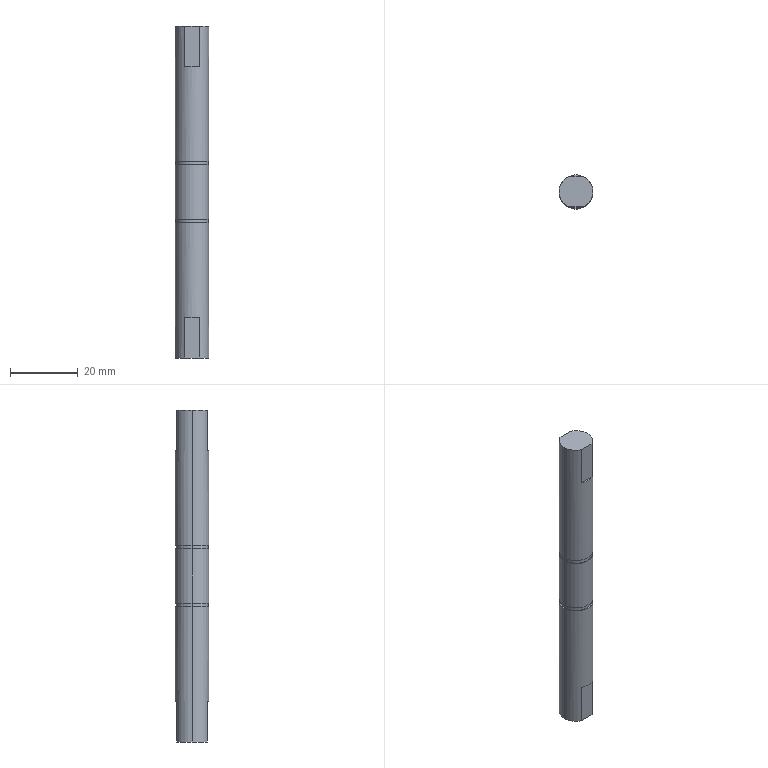Part | SolidWorks | features ICE 2, MirrorPattern 2, Extrusion 1, RefAxis 1 | 1 solid | 24 faces | box 10 x 10 x 98 mm | volume 7613 mm3 | plane 14 | cylinder 10 | commonest cylinder face diameters 10 x6 9.6 x4
STEP:
#1=CARTESIAN_POINT('',(4.8,0.,-9.1));
#2=VERTEX_POINT('',#1);
#3=CARTESIAN_POINT('',(-4.8,0.,-9.1));
#4=VERTEX_POINT('',#3);
#5=CARTESIAN_POINT('',(0.,0.,-9.1));
#6=DIRECTION('',(0.,0.,1.));
#7=DIRECTION('',(1.,0.,0.));
#8=AXIS2_PLACEMENT_3D('',#5,#6,#7);
#9=CIRCLE('',#8,4.8);
#10=EDGE_CURVE('',#2,#4,#9,.T.);
#11=ORIENTED_EDGE('',*,*,#10,.T.);
#12=CARTESIAN_POINT('',(-4.8,0.,-8.));
#13=VERTEX_POINT('',#12);
#14=CARTESIAN_POINT('',(-4.8,0.,-9.1));
#15=DIRECTION('',(0.,0.,1.));
#16=VECTOR('',#15,1000.);
#17=LINE('',#14,#16);
#18=EDGE_CURVE('',#4,#13,#17,.T.);
#19=ORIENTED_EDGE('',*,*,#18,.T.);
#20=CARTESIAN_POINT('',(4.8,0.,-8.));
#21=VERTEX_POINT('',#20);
#22=CARTESIAN_POINT('',(0.,0.,-8.));
#23=DIRECTION('',(0.,0.,1.));
#24=DIRECTION('',(1.,0.,0.));
#25=AXIS2_PLACEMENT_3D('',#22,#23,#24);
#26=CIRCLE('',#25,4.8);
#27=EDGE_CURVE('',#21,#13,#26,.T.);
#28=ORIENTED_EDGE('',*,*,#27,.F.);
#29=CARTESIAN_POINT('',(4.8,0.,-9.1));
#30=DIRECTION('',(0.,0.,1.));
#31=VECTOR('',#30,1000.);
#32=LINE('',#29,#31);
#33=EDGE_CURVE('',#2,#21,#32,.T.);
#34=ORIENTED_EDGE('',*,*,#33,.F.);
#35=EDGE_LOOP('',(#11,#19,#28,#34));
#36=FACE_OUTER_BOUND('',#35,.T.);
#37=CARTESIAN_POINT('',(0.,0.,-9.1));
#38=DIRECTION('',(0.,0.,1.));
#39=DIRECTION('',(1.,0.,0.));
#40=AXIS2_PLACEMENT_3D('',#37,#38,#39);
#41=CYLINDRICAL_SURFACE('',#40,4.8);
#42=ADVANCED_FACE('',(#36),#41,.T.);
#43=CARTESIAN_POINT('',(4.8,0.,9.1));
#44=VERTEX_POINT('',#43);
#45=CARTESIAN_POINT('',(-4.8,0.,9.1));
#46=VERTEX_POINT('',#45);
#47=CARTESIAN_POINT('',(0.,0.,9.1));
#48=DIRECTION('',(0.,0.,1.));
#49=DIRECTION('',(1.,0.,0.));
#50=AXIS2_PLACEMENT_3D('',#47,#48,#49);
#51=CIRCLE('',#50,4.8);
#52=EDGE_CURVE('',#44,#46,#51,.T.);
#53=ORIENTED_EDGE('',*,*,#52,.F.);
#54=CARTESIAN_POINT('',(4.8,0.,8.));
#55=VERTEX_POINT('',#54);
#56=CARTESIAN_POINT('',(4.8,0.,9.1));
#57=DIRECTION('',(0.,0.,-1.));
#58=VECTOR('',#57,1000.);
#59=LINE('',#56,#58);
#60=EDGE_CURVE('',#44,#55,#59,.T.);
#61=ORIENTED_EDGE('',*,*,#60,.T.);
#62=CARTESIAN_POINT('',(-4.8,0.,8.));
#63=VERTEX_POINT('',#62);
#64=CARTESIAN_POINT('',(0.,0.,8.));
#65=DIRECTION('',(0.,0.,1.));
#66=DIRECTION('',(1.,0.,0.));
#67=AXIS2_PLACEMENT_3D('',#64,#65,#66);
#68=CIRCLE('',#67,4.8);
#69=EDGE_CURVE('',#55,#63,#68,.T.);
#70=ORIENTED_EDGE('',*,*,#69,.T.);
#71=CARTESIAN_POINT('',(-4.8,0.,9.1));
#72=DIRECTION('',(0.,0.,-1.));
#73=VECTOR('',#72,1000.);
#74=LINE('',#71,#73);
#75=EDGE_CURVE('',#46,#63,#74,.T.);
#76=ORIENTED_EDGE('',*,*,#75,.F.);
#77=EDGE_LOOP('',(#53,#61,#70,#76));
#78=FACE_OUTER_BOUND('',#77,.T.);
#79=CARTESIAN_POINT('',(0.,0.,9.1));
#80=DIRECTION('',(0.,0.,-1.));
#81=DIRECTION('',(-1.,0.,0.));
#82=AXIS2_PLACEMENT_3D('',#79,#80,#81);
#83=CYLINDRICAL_SURFACE('',#82,4.8);
#84=ADVANCED_FACE('',(#78),#83,.T.);
#85=CARTESIAN_POINT('',(5.,0.,49.));
#86=VERTEX_POINT('',#85);
#87=CARTESIAN_POINT('',(2.179,4.5,49.));
#88=VERTEX_POINT('',#87);
#89=CARTESIAN_POINT('',(0.,0.,49.));
#90=DIRECTION('',(0.,0.,1.));
#91=DIRECTION('',(1.,0.,0.));
#92=AXIS2_PLACEMENT_3D('',#89,#90,#91);
#93=CIRCLE('',#92,5.);
#94=EDGE_CURVE('',#86,#88,#93,.T.);
#95=ORIENTED_EDGE('',*,*,#94,.F.);
#96=CARTESIAN_POINT('',(5.,0.,9.1));
#97=VERTEX_POINT('',#96);
#98=CARTESIAN_POINT('',(5.,0.,49.));
#99=DIRECTION('',(0.,0.,-1.));
#100=VECTOR('',#99,1000.);
#101=LINE('',#98,#100);
#102=EDGE_CURVE('',#86,#97,#101,.T.);
#103=ORIENTED_EDGE('',*,*,#102,.T.);
#104=CARTESIAN_POINT('',(-5.,0.,9.1));
#105=VERTEX_POINT('',#104);
#106=CARTESIAN_POINT('',(0.,0.,9.1));
#107=DIRECTION('',(0.,0.,1.));
#108=DIRECTION('',(1.,0.,0.));
#109=AXIS2_PLACEMENT_3D('',#106,#107,#108);
#110=CIRCLE('',#109,5.);
#111=EDGE_CURVE('',#97,#105,#110,.T.);
#112=ORIENTED_EDGE('',*,*,#111,.T.);
#113=CARTESIAN_POINT('',(-5.,0.,49.));
#114=VERTEX_POINT('',#113);
#115=CARTESIAN_POINT('',(-5.,0.,49.));
#116=DIRECTION('',(0.,0.,-1.));
#117=VECTOR('',#116,1000.);
#118=LINE('',#115,#117);
#119=EDGE_CURVE('',#114,#105,#118,.T.);
#120=ORIENTED_EDGE('',*,*,#119,.F.);
#121=CARTESIAN_POINT('',(-2.179,4.5,49.));
#122=VERTEX_POINT('',#121);
#123=CARTESIAN_POINT('',(0.,0.,49.));
#124=DIRECTION('',(0.,0.,1.));
#125=DIRECTION('',(1.,0.,0.));
#126=AXIS2_PLACEMENT_3D('',#123,#124,#125);
#127=CIRCLE('',#126,5.);
#128=EDGE_CURVE('',#122,#114,#127,.T.);
#129=ORIENTED_EDGE('',*,*,#128,.F.);
#130=CARTESIAN_POINT('',(-2.179,4.5,37.));
#131=VERTEX_POINT('',#130);
#132=CARTESIAN_POINT('',(-2.179,4.5,37.));
#133=DIRECTION('',(0.,0.,1.));
#134=VECTOR('',#133,1000.);
#135=LINE('',#132,#134);
#136=EDGE_CURVE('',#131,#122,#135,.T.);
#137=ORIENTED_EDGE('',*,*,#136,.F.);
#138=CARTESIAN_POINT('',(2.179,4.5,37.));
#139=VERTEX_POINT('',#138);
#140=CARTESIAN_POINT('',(0.,0.,37.));
#141=DIRECTION('',(0.,0.,1.));
#142=DIRECTION('',(1.,0.,0.));
#143=AXIS2_PLACEMENT_3D('',#140,#141,#142);
#144=CIRCLE('',#143,5.);
#145=EDGE_CURVE('',#139,#131,#144,.T.);
#146=ORIENTED_EDGE('',*,*,#145,.F.);
#147=CARTESIAN_POINT('',(2.179,4.5,37.));
#148=DIRECTION('',(0.,0.,1.));
#149=VECTOR('',#148,1000.);
#150=LINE('',#147,#149);
#151=EDGE_CURVE('',#139,#88,#150,.T.);
#152=ORIENTED_EDGE('',*,*,#151,.T.);
#153=EDGE_LOOP('',(#95,#103,#112,#120,#129,#137,#146,#152));
#154=FACE_OUTER_BOUND('',#153,.T.);
#155=CARTESIAN_POINT('',(0.,0.,49.));
#156=DIRECTION('',(0.,0.,-1.));
#157=DIRECTION('',(-1.,0.,0.));
#158=AXIS2_PLACEMENT_3D('',#155,#156,#157);
#159=CYLINDRICAL_SURFACE('',#158,5.);
#160=ADVANCED_FACE('',(#154),#159,.T.);
#161=CARTESIAN_POINT('',(5.,0.,8.));
#162=VERTEX_POINT('',#161);
#163=CARTESIAN_POINT('',(-5.,0.,8.));
#164=VERTEX_POINT('',#163);
#165=CARTESIAN_POINT('',(0.,0.,8.));
#166=DIRECTION('',(0.,0.,1.));
#167=DIRECTION('',(1.,0.,0.));
#168=AXIS2_PLACEMENT_3D('',#165,#166,#167);
#169=CIRCLE('',#168,5.);
#170=EDGE_CURVE('',#162,#164,#169,.T.);
#171=ORIENTED_EDGE('',*,*,#170,.F.);
#172=CARTESIAN_POINT('',(5.,0.,-8.));
#173=VERTEX_POINT('',#172);
#174=CARTESIAN_POINT('',(5.,0.,49.));
#175=DIRECTION('',(0.,0.,-1.));
#176=VECTOR('',#175,1000.);
#177=LINE('',#174,#176);
#178=EDGE_CURVE('',#162,#173,#177,.T.);
#179=ORIENTED_EDGE('',*,*,#178,.T.);
#180=CARTESIAN_POINT('',(-5.,0.,-8.));
#181=VERTEX_POINT('',#180);
#182=CARTESIAN_POINT('',(0.,0.,-8.));
#183=DIRECTION('',(0.,0.,1.));
#184=DIRECTION('',(1.,0.,0.));
#185=AXIS2_PLACEMENT_3D('',#182,#183,#184);
#186=CIRCLE('',#185,5.);
#187=EDGE_CURVE('',#173,#181,#186,.T.);
#188=ORIENTED_EDGE('',*,*,#187,.T.);
#189=CARTESIAN_POINT('',(-5.,0.,49.));
#190=DIRECTION('',(0.,0.,-1.));
#191=VECTOR('',#190,1000.);
#192=LINE('',#189,#191);
#193=EDGE_CURVE('',#164,#181,#192,.T.);
#194=ORIENTED_EDGE('',*,*,#193,.F.);
#195=EDGE_LOOP('',(#171,#179,#188,#194));
#196=FACE_OUTER_BOUND('',#195,.T.);
#197=CARTESIAN_POINT('',(0.,0.,49.));
#198=DIRECTION('',(0.,0.,-1.));
#199=DIRECTION('',(-1.,0.,0.));
#200=AXIS2_PLACEMENT_3D('',#197,#198,#199);
#201=CYLINDRICAL_SURFACE('',#200,5.);
#202=ADVANCED_FACE('',(#196),#201,.T.);
#203=CARTESIAN_POINT('',(5.,0.,-9.1));
#204=VERTEX_POINT('',#203);
#205=CARTESIAN_POINT('',(-5.,0.,-9.1));
#206=VERTEX_POINT('',#205);
#207=CARTESIAN_POINT('',(0.,0.,-9.1));
#208=DIRECTION('',(0.,0.,1.));
#209=DIRECTION('',(1.,0.,0.));
#210=AXIS2_PLACEMENT_3D('',#207,#208,#209);
#211=CIRCLE('',#210,5.);
#212=EDGE_CURVE('',#204,#206,#211,.T.);
#213=ORIENTED_EDGE('',*,*,#212,.F.);
#214=CARTESIAN_POINT('',(5.,0.,-49.));
#215=VERTEX_POINT('',#214);
#216=CARTESIAN_POINT('',(5.,0.,49.));
#217=DIRECTION('',(0.,0.,-1.));
#218=VECTOR('',#217,1000.);
#219=LINE('',#216,#218);
#220=EDGE_CURVE('',#204,#215,#219,.T.);
#221=ORIENTED_EDGE('',*,*,#220,.T.);
#222=CARTESIAN_POINT('',(2.179,4.5,-49.));
#223=VERTEX_POINT('',#222);
#224=CARTESIAN_POINT('',(0.,0.,-49.));
#225=DIRECTION('',(0.,0.,1.));
#226=DIRECTION('',(1.,0.,0.));
#227=AXIS2_PLACEMENT_3D('',#224,#225,#226);
#228=CIRCLE('',#227,5.);
#229=EDGE_CURVE('',#215,#223,#228,.T.);
#230=ORIENTED_EDGE('',*,*,#229,.T.);
#231=CARTESIAN_POINT('',(2.179,4.5,-37.));
#232=VERTEX_POINT('',#231);
#233=CARTESIAN_POINT('',(2.179,4.5,-37.));
#234=DIRECTION('',(0.,0.,-1.));
#235=VECTOR('',#234,1000.);
#236=LINE('',#233,#235);
#237=EDGE_CURVE('',#232,#223,#236,.T.);
#238=ORIENTED_EDGE('',*,*,#237,.F.);
#239=CARTESIAN_POINT('',(-2.179,4.5,-37.));
#240=VERTEX_POINT('',#239);
#241=CARTESIAN_POINT('',(0.,0.,-37.));
#242=DIRECTION('',(0.,0.,1.));
#243=DIRECTION('',(1.,0.,0.));
#244=AXIS2_PLACEMENT_3D('',#241,#242,#243);
#245=CIRCLE('',#244,5.);
#246=EDGE_CURVE('',#232,#240,#245,.T.);
#247=ORIENTED_EDGE('',*,*,#246,.T.);
#248=CARTESIAN_POINT('',(-2.179,4.5,-49.));
#249=VERTEX_POINT('',#248);
#250=CARTESIAN_POINT('',(-2.179,4.5,-37.));
#251=DIRECTION('',(0.,0.,-1.));
#252=VECTOR('',#251,1000.);
#253=LINE('',#250,#252);
#254=EDGE_CURVE('',#240,#249,#253,.T.);
#255=ORIENTED_EDGE('',*,*,#254,.T.);
#256=CARTESIAN_POINT('',(-5.,0.,-49.));
#257=VERTEX_POINT('',#256);
#258=CARTESIAN_POINT('',(0.,0.,-49.));
#259=DIRECTION('',(0.,0.,1.));
#260=DIRECTION('',(1.,0.,0.));
#261=AXIS2_PLACEMENT_3D('',#258,#259,#260);
#262=CIRCLE('',#261,5.);
#263=EDGE_CURVE('',#249,#257,#262,.T.);
#264=ORIENTED_EDGE('',*,*,#263,.T.);
#265=CARTESIAN_POINT('',(-5.,0.,49.));
#266=DIRECTION('',(0.,0.,-1.));
#267=VECTOR('',#266,1000.);
#268=LINE('',#265,#267);
#269=EDGE_CURVE('',#206,#257,#268,.T.);
#270=ORIENTED_EDGE('',*,*,#269,.F.);
#271=EDGE_LOOP('',(#213,#221,#230,#238,#247,#255,#264,#270));
#272=FACE_OUTER_BOUND('',#271,.T.);
#273=CARTESIAN_POINT('',(0.,0.,49.));
#274=DIRECTION('',(0.,0.,-1.));
#275=DIRECTION('',(-1.,0.,0.));
#276=AXIS2_PLACEMENT_3D('',#273,#274,#275);
#277=CYLINDRICAL_SURFACE('',#276,5.);
#278=ADVANCED_FACE('',(#272),#277,.T.);
#279=CARTESIAN_POINT('',(-2.179,4.5,-49.));
#280=DIRECTION('',(1.,0.,0.));
#281=VECTOR('',#280,1000.);
#282=LINE('',#279,#281);
#283=EDGE_CURVE('',#249,#223,#282,.T.);
#284=ORIENTED_EDGE('',*,*,#283,.T.);
#285=ORIENTED_EDGE('',*,*,#229,.F.);
#286=CARTESIAN_POINT('',(2.179,-4.5,-49.));
#287=VERTEX_POINT('',#286);
#288=CARTESIAN_POINT('',(0.,0.,-49.));
#289=DIRECTION('',(0.,0.,1.));
#290=DIRECTION('',(1.,0.,0.));
#291=AXIS2_PLACEMENT_3D('',#288,#289,#290);
#292=CIRCLE('',#291,5.);
#293=EDGE_CURVE('',#287,#215,#292,.T.);
#294=ORIENTED_EDGE('',*,*,#293,.F.);
#295=CARTESIAN_POINT('',(-2.179,-4.5,-49.));
#296=VERTEX_POINT('',#295);
#297=CARTESIAN_POINT('',(-2.179,-4.5,-49.));
#298=DIRECTION('',(-1.,0.,0.));
#299=VECTOR('',#298,1000.);
#300=LINE('',#297,#299);
#301=EDGE_CURVE('',#287,#296,#300,.T.);
#302=ORIENTED_EDGE('',*,*,#301,.T.);
#303=CARTESIAN_POINT('',(0.,0.,-49.));
#304=DIRECTION('',(0.,0.,1.));
#305=DIRECTION('',(1.,0.,0.));
#306=AXIS2_PLACEMENT_3D('',#303,#304,#305);
#307=CIRCLE('',#306,5.);
#308=EDGE_CURVE('',#257,#296,#307,.T.);
#309=ORIENTED_EDGE('',*,*,#308,.F.);
#310=ORIENTED_EDGE('',*,*,#263,.F.);
#311=EDGE_LOOP('',(#284,#285,#294,#302,#309,#310));
#312=FACE_OUTER_BOUND('',#311,.T.);
#313=CARTESIAN_POINT('',(0.,0.,-49.));
#314=DIRECTION('',(0.,0.,1.));
#315=DIRECTION('',(1.,0.,0.));
#316=AXIS2_PLACEMENT_3D('',#313,#314,#315);
#317=PLANE('',#316);
#318=ADVANCED_FACE('',(#312),#317,.F.);
#319=ORIENTED_EDGE('',*,*,#220,.F.);
#320=CARTESIAN_POINT('',(0.,0.,-9.1));
#321=DIRECTION('',(0.,0.,1.));
#322=DIRECTION('',(1.,0.,0.));
#323=AXIS2_PLACEMENT_3D('',#320,#321,#322);
#324=CIRCLE('',#323,5.);
#325=EDGE_CURVE('',#206,#204,#324,.T.);
#326=ORIENTED_EDGE('',*,*,#325,.F.);
#327=ORIENTED_EDGE('',*,*,#269,.T.);
#328=ORIENTED_EDGE('',*,*,#308,.T.);
#329=CARTESIAN_POINT('',(-2.179,-4.5,-37.));
#330=VERTEX_POINT('',#329);
#331=CARTESIAN_POINT('',(-2.179,-4.5,-37.));
#332=DIRECTION('',(0.,0.,-1.));
#333=VECTOR('',#332,1000.);
#334=LINE('',#331,#333);
#335=EDGE_CURVE('',#330,#296,#334,.T.);
#336=ORIENTED_EDGE('',*,*,#335,.F.);
#337=CARTESIAN_POINT('',(2.179,-4.5,-37.));
#338=VERTEX_POINT('',#337);
#339=CARTESIAN_POINT('',(0.,0.,-37.));
#340=DIRECTION('',(0.,0.,1.));
#341=DIRECTION('',(1.,0.,0.));
#342=AXIS2_PLACEMENT_3D('',#339,#340,#341);
#343=CIRCLE('',#342,5.);
#344=EDGE_CURVE('',#330,#338,#343,.T.);
#345=ORIENTED_EDGE('',*,*,#344,.T.);
#346=CARTESIAN_POINT('',(2.179,-4.5,-37.));
#347=DIRECTION('',(0.,0.,-1.));
#348=VECTOR('',#347,1000.);
#349=LINE('',#346,#348);
#350=EDGE_CURVE('',#338,#287,#349,.T.);
#351=ORIENTED_EDGE('',*,*,#350,.T.);
#352=ORIENTED_EDGE('',*,*,#293,.T.);
#353=EDGE_LOOP('',(#319,#326,#327,#328,#336,#345,#351,#352));
#354=FACE_OUTER_BOUND('',#353,.T.);
#355=CARTESIAN_POINT('',(0.,0.,49.));
#356=DIRECTION('',(0.,0.,-1.));
#357=DIRECTION('',(-1.,0.,0.));
#358=AXIS2_PLACEMENT_3D('',#355,#356,#357);
#359=CYLINDRICAL_SURFACE('',#358,5.);
#360=ADVANCED_FACE('',(#354),#359,.T.);
#361=ORIENTED_EDGE('',*,*,#178,.F.);
#362=CARTESIAN_POINT('',(0.,0.,8.));
#363=DIRECTION('',(0.,0.,1.));
#364=DIRECTION('',(1.,0.,0.));
#365=AXIS2_PLACEMENT_3D('',#362,#363,#364);
#366=CIRCLE('',#365,5.);
#367=EDGE_CURVE('',#164,#162,#366,.T.);
#368=ORIENTED_EDGE('',*,*,#367,.F.);
#369=ORIENTED_EDGE('',*,*,#193,.T.);
#370=CARTESIAN_POINT('',(0.,0.,-8.));
#371=DIRECTION('',(0.,0.,1.));
#372=DIRECTION('',(1.,0.,0.));
#373=AXIS2_PLACEMENT_3D('',#370,#371,#372);
#374=CIRCLE('',#373,5.);
#375=EDGE_CURVE('',#181,#173,#374,.T.);
#376=ORIENTED_EDGE('',*,*,#375,.T.);
#377=EDGE_LOOP('',(#361,#368,#369,#376));
#378=FACE_OUTER_BOUND('',#377,.T.);
#379=CARTESIAN_POINT('',(0.,0.,49.));
#380=DIRECTION('',(0.,0.,-1.));
#381=DIRECTION('',(-1.,0.,0.));
#382=AXIS2_PLACEMENT_3D('',#379,#380,#381);
#383=CYLINDRICAL_SURFACE('',#382,5.);
#384=ADVANCED_FACE('',(#378),#383,.T.);
#385=ORIENTED_EDGE('',*,*,#102,.F.);
#386=CARTESIAN_POINT('',(2.179,-4.5,49.));
#387=VERTEX_POINT('',#386);
#388=CARTESIAN_POINT('',(0.,0.,49.));
#389=DIRECTION('',(0.,0.,1.));
#390=DIRECTION('',(1.,0.,0.));
#391=AXIS2_PLACEMENT_3D('',#388,#389,#390);
#392=CIRCLE('',#391,5.);
#393=EDGE_CURVE('',#387,#86,#392,.T.);
#394=ORIENTED_EDGE('',*,*,#393,.F.);
#395=CARTESIAN_POINT('',(2.179,-4.5,37.));
#396=VERTEX_POINT('',#395);
#397=CARTESIAN_POINT('',(2.179,-4.5,37.));
#398=DIRECTION('',(0.,0.,1.));
#399=VECTOR('',#398,1000.);
#400=LINE('',#397,#399);
#401=EDGE_CURVE('',#396,#387,#400,.T.);
#402=ORIENTED_EDGE('',*,*,#401,.F.);
#403=CARTESIAN_POINT('',(-2.179,-4.5,37.));
#404=VERTEX_POINT('',#403);
#405=CARTESIAN_POINT('',(0.,0.,37.));
#406=DIRECTION('',(0.,0.,1.));
#407=DIRECTION('',(1.,0.,0.));
#408=AXIS2_PLACEMENT_3D('',#405,#406,#407);
#409=CIRCLE('',#408,5.);
#410=EDGE_CURVE('',#404,#396,#409,.T.);
#411=ORIENTED_EDGE('',*,*,#410,.F.);
#412=CARTESIAN_POINT('',(-2.179,-4.5,49.));
#413=VERTEX_POINT('',#412);
#414=CARTESIAN_POINT('',(-2.179,-4.5,37.));
#415=DIRECTION('',(0.,0.,1.));
#416=VECTOR('',#415,1000.);
#417=LINE('',#414,#416);
#418=EDGE_CURVE('',#404,#413,#417,.T.);
#419=ORIENTED_EDGE('',*,*,#418,.T.);
#420=CARTESIAN_POINT('',(0.,0.,49.));
#421=DIRECTION('',(0.,0.,1.));
#422=DIRECTION('',(1.,0.,0.));
#423=AXIS2_PLACEMENT_3D('',#420,#421,#422);
#424=CIRCLE('',#423,5.);
#425=EDGE_CURVE('',#114,#413,#424,.T.);
#426=ORIENTED_EDGE('',*,*,#425,.F.);
#427=ORIENTED_EDGE('',*,*,#119,.T.);
#428=CARTESIAN_POINT('',(0.,0.,9.1));
#429=DIRECTION('',(0.,0.,1.));
#430=DIRECTION('',(1.,0.,0.));
#431=AXIS2_PLACEMENT_3D('',#428,#429,#430);
#432=CIRCLE('',#431,5.);
#433=EDGE_CURVE('',#105,#97,#432,.T.);
#434=ORIENTED_EDGE('',*,*,#433,.T.);
#435=EDGE_LOOP('',(#385,#394,#402,#411,#419,#426,#427,#434));
#436=FACE_OUTER_BOUND('',#435,.T.);
#437=CARTESIAN_POINT('',(0.,0.,49.));
#438=DIRECTION('',(0.,0.,-1.));
#439=DIRECTION('',(-1.,0.,0.));
#440=AXIS2_PLACEMENT_3D('',#437,#438,#439);
#441=CYLINDRICAL_SURFACE('',#440,5.);
#442=ADVANCED_FACE('',(#436),#441,.T.);
#443=CARTESIAN_POINT('',(-2.179,4.5,49.));
#444=DIRECTION('',(1.,0.,0.));
#445=VECTOR('',#444,1000.);
#446=LINE('',#443,#445);
#447=EDGE_CURVE('',#122,#88,#446,.T.);
#448=ORIENTED_EDGE('',*,*,#447,.F.);
#449=ORIENTED_EDGE('',*,*,#128,.T.);
#450=ORIENTED_EDGE('',*,*,#425,.T.);
#451=CARTESIAN_POINT('',(-2.179,-4.5,49.));
#452=DIRECTION('',(-1.,0.,0.));
#453=VECTOR('',#452,1000.);
#454=LINE('',#451,#453);
#455=EDGE_CURVE('',#387,#413,#454,.T.);
#456=ORIENTED_EDGE('',*,*,#455,.F.);
#457=ORIENTED_EDGE('',*,*,#393,.T.);
#458=ORIENTED_EDGE('',*,*,#94,.T.);
#459=EDGE_LOOP('',(#448,#449,#450,#456,#457,#458));
#460=FACE_OUTER_BOUND('',#459,.T.);
#461=CARTESIAN_POINT('',(0.,0.,49.));
#462=DIRECTION('',(0.,0.,1.));
#463=DIRECTION('',(1.,0.,0.));
#464=AXIS2_PLACEMENT_3D('',#461,#462,#463);
#465=PLANE('',#464);
#466=ADVANCED_FACE('',(#460),#465,.T.);
#467=ORIENTED_EDGE('',*,*,#433,.F.);
#468=ORIENTED_EDGE('',*,*,#111,.F.);
#469=EDGE_LOOP('',(#467,#468));
#470=FACE_OUTER_BOUND('',#469,.T.);
#471=CARTESIAN_POINT('',(0.,0.,9.1));
#472=DIRECTION('',(0.,0.,1.));
#473=DIRECTION('',(1.,0.,0.));
#474=AXIS2_PLACEMENT_3D('',#471,#472,#473);
#475=CIRCLE('',#474,4.8);
#476=EDGE_CURVE('',#46,#44,#475,.T.);
#477=ORIENTED_EDGE('',*,*,#476,.T.);
#478=ORIENTED_EDGE('',*,*,#52,.T.);
#479=EDGE_LOOP('',(#477,#478));
#480=FACE_BOUND('',#479,.T.);
#481=CARTESIAN_POINT('',(0.,0.,9.1));
#482=DIRECTION('',(0.,0.,1.));
#483=DIRECTION('',(1.,0.,0.));
#484=AXIS2_PLACEMENT_3D('',#481,#482,#483);
#485=PLANE('',#484);
#486=ADVANCED_FACE('',(#470,#480),#485,.F.);
#487=ORIENTED_EDGE('',*,*,#367,.T.);
#488=ORIENTED_EDGE('',*,*,#170,.T.);
#489=EDGE_LOOP('',(#487,#488));
#490=FACE_OUTER_BOUND('',#489,.T.);
#491=CARTESIAN_POINT('',(0.,0.,8.));
#492=DIRECTION('',(0.,0.,1.));
#493=DIRECTION('',(1.,0.,0.));
#494=AXIS2_PLACEMENT_3D('',#491,#492,#493);
#495=CIRCLE('',#494,4.8);
#496=EDGE_CURVE('',#63,#55,#495,.T.);
#497=ORIENTED_EDGE('',*,*,#496,.F.);
#498=ORIENTED_EDGE('',*,*,#69,.F.);
#499=EDGE_LOOP('',(#497,#498));
#500=FACE_BOUND('',#499,.T.);
#501=CARTESIAN_POINT('',(0.,0.,8.));
#502=DIRECTION('',(0.,0.,1.));
#503=DIRECTION('',(1.,0.,0.));
#504=AXIS2_PLACEMENT_3D('',#501,#502,#503);
#505=PLANE('',#504);
#506=ADVANCED_FACE('',(#490,#500),#505,.T.);
#507=ORIENTED_EDGE('',*,*,#60,.F.);
#508=ORIENTED_EDGE('',*,*,#476,.F.);
#509=ORIENTED_EDGE('',*,*,#75,.T.);
#510=ORIENTED_EDGE('',*,*,#496,.T.);
#511=EDGE_LOOP('',(#507,#508,#509,#510));
#512=FACE_OUTER_BOUND('',#511,.T.);
#513=CARTESIAN_POINT('',(0.,0.,9.1));
#514=DIRECTION('',(0.,0.,-1.));
#515=DIRECTION('',(-1.,0.,0.));
#516=AXIS2_PLACEMENT_3D('',#513,#514,#515);
#517=CYLINDRICAL_SURFACE('',#516,4.8);
#518=ADVANCED_FACE('',(#512),#517,.T.);
#519=ORIENTED_EDGE('',*,*,#10,.F.);
#520=CARTESIAN_POINT('',(0.,0.,-9.1));
#521=DIRECTION('',(0.,0.,1.));
#522=DIRECTION('',(1.,0.,0.));
#523=AXIS2_PLACEMENT_3D('',#520,#521,#522);
#524=CIRCLE('',#523,4.8);
#525=EDGE_CURVE('',#4,#2,#524,.T.);
#526=ORIENTED_EDGE('',*,*,#525,.F.);
#527=EDGE_LOOP('',(#519,#526));
#528=FACE_BOUND('',#527,.T.);
#529=ORIENTED_EDGE('',*,*,#325,.T.);
#530=ORIENTED_EDGE('',*,*,#212,.T.);
#531=EDGE_LOOP('',(#529,#530));
#532=FACE_OUTER_BOUND('',#531,.T.);
#533=CARTESIAN_POINT('',(0.,0.,-9.1));
#534=DIRECTION('',(0.,0.,-1.));
#535=DIRECTION('',(1.,0.,0.));
#536=AXIS2_PLACEMENT_3D('',#533,#534,#535);
#537=PLANE('',#536);
#538=ADVANCED_FACE('',(#528,#532),#537,.F.);
#539=ORIENTED_EDGE('',*,*,#27,.T.);
#540=CARTESIAN_POINT('',(0.,0.,-8.));
#541=DIRECTION('',(0.,0.,1.));
#542=DIRECTION('',(1.,0.,0.));
#543=AXIS2_PLACEMENT_3D('',#540,#541,#542);
#544=CIRCLE('',#543,4.8);
#545=EDGE_CURVE('',#13,#21,#544,.T.);
#546=ORIENTED_EDGE('',*,*,#545,.T.);
#547=EDGE_LOOP('',(#539,#546));
#548=FACE_BOUND('',#547,.T.);
#549=ORIENTED_EDGE('',*,*,#375,.F.);
#550=ORIENTED_EDGE('',*,*,#187,.F.);
#551=EDGE_LOOP('',(#549,#550));
#552=FACE_OUTER_BOUND('',#551,.T.);
#553=CARTESIAN_POINT('',(0.,0.,-8.));
#554=DIRECTION('',(0.,0.,-1.));
#555=DIRECTION('',(1.,0.,0.));
#556=AXIS2_PLACEMENT_3D('',#553,#554,#555);
#557=PLANE('',#556);
#558=ADVANCED_FACE('',(#548,#552),#557,.T.);
#559=ORIENTED_EDGE('',*,*,#18,.F.);
#560=ORIENTED_EDGE('',*,*,#525,.T.);
#561=ORIENTED_EDGE('',*,*,#33,.T.);
#562=ORIENTED_EDGE('',*,*,#545,.F.);
#563=EDGE_LOOP('',(#559,#560,#561,#562));
#564=FACE_OUTER_BOUND('',#563,.T.);
#565=CARTESIAN_POINT('',(0.,0.,-9.1));
#566=DIRECTION('',(0.,0.,1.));
#567=DIRECTION('',(1.,0.,0.));
#568=AXIS2_PLACEMENT_3D('',#565,#566,#567);
#569=CYLINDRICAL_SURFACE('',#568,4.8);
#570=ADVANCED_FACE('',(#564),#569,.T.);
#571=ORIENTED_EDGE('',*,*,#455,.T.);
#572=ORIENTED_EDGE('',*,*,#418,.F.);
#573=CARTESIAN_POINT('',(-2.179,-4.5,37.));
#574=DIRECTION('',(-1.,0.,0.));
#575=VECTOR('',#574,1000.);
#576=LINE('',#573,#575);
#577=EDGE_CURVE('',#396,#404,#576,.T.);
#578=ORIENTED_EDGE('',*,*,#577,.F.);
#579=ORIENTED_EDGE('',*,*,#401,.T.);
#580=EDGE_LOOP('',(#571,#572,#578,#579));
#581=FACE_OUTER_BOUND('',#580,.T.);
#582=CARTESIAN_POINT('',(-2.179,-4.5,37.));
#583=DIRECTION('',(0.,1.,0.));
#584=DIRECTION('',(0.,0.,1.));
#585=AXIS2_PLACEMENT_3D('',#582,#583,#584);
#586=PLANE('',#585);
#587=ADVANCED_FACE('',(#581),#586,.F.);
#588=ORIENTED_EDGE('',*,*,#410,.T.);
#589=ORIENTED_EDGE('',*,*,#577,.T.);
#590=EDGE_LOOP('',(#588,#589));
#591=FACE_OUTER_BOUND('',#590,.T.);
#592=CARTESIAN_POINT('',(0.,0.,37.));
#593=DIRECTION('',(0.,0.,1.));
#594=DIRECTION('',(1.,0.,0.));
#595=AXIS2_PLACEMENT_3D('',#592,#593,#594);
#596=PLANE('',#595);
#597=ADVANCED_FACE('',(#591),#596,.T.);
#598=ORIENTED_EDGE('',*,*,#447,.T.);
#599=ORIENTED_EDGE('',*,*,#151,.F.);
#600=CARTESIAN_POINT('',(-2.179,4.5,37.));
#601=DIRECTION('',(1.,0.,0.));
#602=VECTOR('',#601,1000.);
#603=LINE('',#600,#602);
#604=EDGE_CURVE('',#131,#139,#603,.T.);
#605=ORIENTED_EDGE('',*,*,#604,.F.);
#606=ORIENTED_EDGE('',*,*,#136,.T.);
#607=EDGE_LOOP('',(#598,#599,#605,#606));
#608=FACE_OUTER_BOUND('',#607,.T.);
#609=CARTESIAN_POINT('',(-2.179,4.5,37.));
#610=DIRECTION('',(0.,-1.,0.));
#611=DIRECTION('',(0.,0.,-1.));
#612=AXIS2_PLACEMENT_3D('',#609,#610,#611);
#613=PLANE('',#612);
#614=ADVANCED_FACE('',(#608),#613,.F.);
#615=ORIENTED_EDGE('',*,*,#145,.T.);
#616=ORIENTED_EDGE('',*,*,#604,.T.);
#617=EDGE_LOOP('',(#615,#616));
#618=FACE_OUTER_BOUND('',#617,.T.);
#619=CARTESIAN_POINT('',(0.,0.,37.));
#620=DIRECTION('',(0.,0.,1.));
#621=DIRECTION('',(1.,0.,0.));
#622=AXIS2_PLACEMENT_3D('',#619,#620,#621);
#623=PLANE('',#622);
#624=ADVANCED_FACE('',(#618),#623,.T.);
#625=ORIENTED_EDGE('',*,*,#301,.F.);
#626=ORIENTED_EDGE('',*,*,#350,.F.);
#627=CARTESIAN_POINT('',(-2.179,-4.5,-37.));
#628=DIRECTION('',(-1.,0.,0.));
#629=VECTOR('',#628,1000.);
#630=LINE('',#627,#629);
#631=EDGE_CURVE('',#338,#330,#630,.T.);
#632=ORIENTED_EDGE('',*,*,#631,.T.);
#633=ORIENTED_EDGE('',*,*,#335,.T.);
#634=EDGE_LOOP('',(#625,#626,#632,#633));
#635=FACE_OUTER_BOUND('',#634,.T.);
#636=CARTESIAN_POINT('',(-2.179,-4.5,-37.));
#637=DIRECTION('',(0.,-1.,0.));
#638=DIRECTION('',(0.,0.,-1.));
#639=AXIS2_PLACEMENT_3D('',#636,#637,#638);
#640=PLANE('',#639);
#641=ADVANCED_FACE('',(#635),#640,.T.);
#642=ORIENTED_EDGE('',*,*,#344,.F.);
#643=ORIENTED_EDGE('',*,*,#631,.F.);
#644=EDGE_LOOP('',(#642,#643));
#645=FACE_OUTER_BOUND('',#644,.T.);
#646=CARTESIAN_POINT('',(0.,0.,-37.));
#647=DIRECTION('',(0.,0.,-1.));
#648=DIRECTION('',(1.,0.,0.));
#649=AXIS2_PLACEMENT_3D('',#646,#647,#648);
#650=PLANE('',#649);
#651=ADVANCED_FACE('',(#645),#650,.T.);
#652=ORIENTED_EDGE('',*,*,#283,.F.);
#653=ORIENTED_EDGE('',*,*,#254,.F.);
#654=CARTESIAN_POINT('',(-2.179,4.5,-37.));
#655=DIRECTION('',(1.,0.,0.));
#656=VECTOR('',#655,1000.);
#657=LINE('',#654,#656);
#658=EDGE_CURVE('',#240,#232,#657,.T.);
#659=ORIENTED_EDGE('',*,*,#658,.T.);
#660=ORIENTED_EDGE('',*,*,#237,.T.);
#661=EDGE_LOOP('',(#652,#653,#659,#660));
#662=FACE_OUTER_BOUND('',#661,.T.);
#663=CARTESIAN_POINT('',(-2.179,4.5,-37.));
#664=DIRECTION('',(0.,1.,0.));
#665=DIRECTION('',(0.,0.,1.));
#666=AXIS2_PLACEMENT_3D('',#663,#664,#665);
#667=PLANE('',#666);
#668=ADVANCED_FACE('',(#662),#667,.T.);
#669=ORIENTED_EDGE('',*,*,#246,.F.);
#670=ORIENTED_EDGE('',*,*,#658,.F.);
#671=EDGE_LOOP('',(#669,#670));
#672=FACE_OUTER_BOUND('',#671,.T.);
#673=CARTESIAN_POINT('',(0.,0.,-37.));
#674=DIRECTION('',(0.,0.,-1.));
#675=DIRECTION('',(1.,0.,0.));
#676=AXIS2_PLACEMENT_3D('',#673,#674,#675);
#677=PLANE('',#676);
#678=ADVANCED_FACE('',(#672),#677,.T.);
#679=CLOSED_SHELL('',(#42,#84,#160,#202,#278,#318,#360,#384,#442,#466,#486,#506,#518,#538,#558,#570,#587,#597,#614,#624,#641,#651,#668,#678));
#680=MANIFOLD_SOLID_BREP('',#679);
#681=CARTESIAN_POINT('',(0.,0.,0.));
#682=DIRECTION('',(0.,0.,1.));
#683=DIRECTION('',(1.,0.,0.));
#684=AXIS2_PLACEMENT_3D('',#681,#682,#683);
#685=(LENGTH_UNIT()NAMED_UNIT(*)SI_UNIT(.MILLI.,.METRE.));
#686=UNCERTAINTY_MEASURE_WITH_UNIT(LENGTH_MEASURE(0.00001),#685,'','');
#687=(NAMED_UNIT(*)PLANE_ANGLE_UNIT()SI_UNIT($,.RADIAN.));
#688=(NAMED_UNIT(*)SI_UNIT($,.STERADIAN.)SOLID_ANGLE_UNIT());
#689=(GEOMETRIC_REPRESENTATION_CONTEXT(3)GLOBAL_UNCERTAINTY_ASSIGNED_CONTEXT((#686))GLOBAL_UNIT_ASSIGNED_CONTEXT((#685,#687,#688))REPRESENTATION_CONTEXT('',''));
#690=ADVANCED_BREP_SHAPE_REPRESENTATION('',(#680,#684),#689);